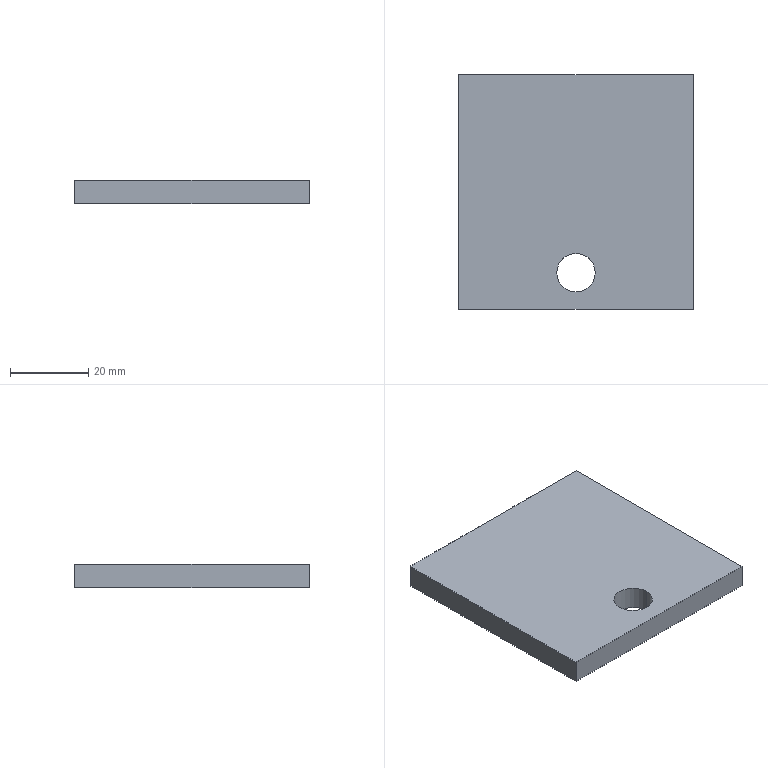Part | NX | features 凸台-拉伸21[2] 2 | 1 solid | 8 faces | box 60 x 60 x 6 mm | volume 21144 mm3 | plane 6 | cylinder 2 | commonest cylinder face diameters 9.834 x2
STEP:
#1=CARTESIAN_POINT('',(2758.083,-50.65,-1102.985));
#2=VERTEX_POINT('',#1);
#3=CARTESIAN_POINT('',(2758.083,-50.65,-1108.985));
#4=VERTEX_POINT('',#3);
#5=CARTESIAN_POINT('',(2758.083,-50.65,-1108.985));
#6=DIRECTION('',(0.,0.,1.));
#7=VECTOR('',#6,1000.);
#8=LINE('',#5,#7);
#9=EDGE_CURVE('',#2,#4,#8,.F.);
#10=ORIENTED_EDGE('',*,*,#9,.T.);
#11=CARTESIAN_POINT('',(2767.917,-50.65,-1108.985));
#12=VERTEX_POINT('',#11);
#13=CARTESIAN_POINT('',(2763.,-50.65,-1108.985));
#14=DIRECTION('',(0.,0.,-1.));
#15=DIRECTION('',(-1.,0.,0.));
#16=AXIS2_PLACEMENT_3D('',#13,#14,#15);
#17=CIRCLE('',#16,4.917);
#18=EDGE_CURVE('',#4,#12,#17,.T.);
#19=ORIENTED_EDGE('',*,*,#18,.T.);
#20=CARTESIAN_POINT('',(2767.917,-50.65,-1102.985));
#21=VERTEX_POINT('',#20);
#22=CARTESIAN_POINT('',(2767.917,-50.65,-1108.985));
#23=DIRECTION('',(0.,0.,1.));
#24=VECTOR('',#23,1000.);
#25=LINE('',#22,#24);
#26=EDGE_CURVE('',#12,#21,#25,.T.);
#27=ORIENTED_EDGE('',*,*,#26,.T.);
#28=CARTESIAN_POINT('',(2763.,-50.65,-1102.985));
#29=DIRECTION('',(0.,0.,-1.));
#30=DIRECTION('',(-1.,0.,0.));
#31=AXIS2_PLACEMENT_3D('',#28,#29,#30);
#32=CIRCLE('',#31,4.917);
#33=EDGE_CURVE('',#2,#21,#32,.T.);
#34=ORIENTED_EDGE('',*,*,#33,.F.);
#35=EDGE_LOOP('',(#10,#19,#27,#34));
#36=FACE_BOUND('',#35,.T.);
#37=CARTESIAN_POINT('',(2763.,-50.65,-1108.985));
#38=DIRECTION('',(0.,0.,1.));
#39=DIRECTION('',(1.,0.,0.));
#40=AXIS2_PLACEMENT_3D('',#37,#38,#39);
#41=CYLINDRICAL_SURFACE('',#40,4.917);
#42=ADVANCED_FACE('',(#36),#41,.F.);
#43=CARTESIAN_POINT('',(2733.,0.,-1102.985));
#44=VERTEX_POINT('',#43);
#45=CARTESIAN_POINT('',(2793.,0.,-1102.985));
#46=VERTEX_POINT('',#45);
#47=CARTESIAN_POINT('',(2793.,0.,-1102.985));
#48=DIRECTION('',(1.,0.,0.));
#49=VECTOR('',#48,1000.);
#50=LINE('',#47,#49);
#51=EDGE_CURVE('',#44,#46,#50,.T.);
#52=ORIENTED_EDGE('',*,*,#51,.T.);
#53=CARTESIAN_POINT('',(2793.,0.,-1108.985));
#54=VERTEX_POINT('',#53);
#55=CARTESIAN_POINT('',(2793.,0.,-1108.985));
#56=DIRECTION('',(0.,0.,1.));
#57=VECTOR('',#56,1000.);
#58=LINE('',#55,#57);
#59=EDGE_CURVE('',#54,#46,#58,.T.);
#60=ORIENTED_EDGE('',*,*,#59,.F.);
#61=CARTESIAN_POINT('',(2733.,0.,-1108.985));
#62=VERTEX_POINT('',#61);
#63=CARTESIAN_POINT('',(2793.,0.,-1108.985));
#64=DIRECTION('',(1.,0.,0.));
#65=VECTOR('',#64,1000.);
#66=LINE('',#63,#65);
#67=EDGE_CURVE('',#62,#54,#66,.T.);
#68=ORIENTED_EDGE('',*,*,#67,.F.);
#69=CARTESIAN_POINT('',(2733.,0.,-1108.985));
#70=DIRECTION('',(0.,0.,1.));
#71=VECTOR('',#70,1000.);
#72=LINE('',#69,#71);
#73=EDGE_CURVE('',#62,#44,#72,.T.);
#74=ORIENTED_EDGE('',*,*,#73,.T.);
#75=EDGE_LOOP('',(#52,#60,#68,#74));
#76=FACE_BOUND('',#75,.T.);
#77=CARTESIAN_POINT('',(2793.,0.,-1108.985));
#78=DIRECTION('',(0.,-1.,0.));
#79=DIRECTION('',(1.,0.,0.));
#80=AXIS2_PLACEMENT_3D('',#77,#78,#79);
#81=PLANE('',#80);
#82=ADVANCED_FACE('',(#76),#81,.F.);
#83=CARTESIAN_POINT('',(2733.,-60.,-1102.985));
#84=VERTEX_POINT('',#83);
#85=CARTESIAN_POINT('',(2733.,0.,-1102.985));
#86=DIRECTION('',(0.,1.,0.));
#87=VECTOR('',#86,1000.);
#88=LINE('',#85,#87);
#89=EDGE_CURVE('',#84,#44,#88,.T.);
#90=ORIENTED_EDGE('',*,*,#89,.T.);
#91=ORIENTED_EDGE('',*,*,#73,.F.);
#92=CARTESIAN_POINT('',(2733.,-60.,-1108.985));
#93=VERTEX_POINT('',#92);
#94=CARTESIAN_POINT('',(2733.,0.,-1108.985));
#95=DIRECTION('',(0.,1.,0.));
#96=VECTOR('',#95,1000.);
#97=LINE('',#94,#96);
#98=EDGE_CURVE('',#93,#62,#97,.T.);
#99=ORIENTED_EDGE('',*,*,#98,.F.);
#100=CARTESIAN_POINT('',(2733.,-60.,-1108.985));
#101=DIRECTION('',(0.,0.,1.));
#102=VECTOR('',#101,1000.);
#103=LINE('',#100,#102);
#104=EDGE_CURVE('',#93,#84,#103,.T.);
#105=ORIENTED_EDGE('',*,*,#104,.T.);
#106=EDGE_LOOP('',(#90,#91,#99,#105));
#107=FACE_BOUND('',#106,.T.);
#108=CARTESIAN_POINT('',(2733.,0.,-1108.985));
#109=DIRECTION('',(1.,0.,0.));
#110=DIRECTION('',(0.,0.,-1.));
#111=AXIS2_PLACEMENT_3D('',#108,#109,#110);
#112=PLANE('',#111);
#113=ADVANCED_FACE('',(#107),#112,.F.);
#114=CARTESIAN_POINT('',(2793.,-60.,-1102.985));
#115=VERTEX_POINT('',#114);
#116=CARTESIAN_POINT('',(2793.,-60.,-1102.985));
#117=DIRECTION('',(-1.,0.,0.));
#118=VECTOR('',#117,1000.);
#119=LINE('',#116,#118);
#120=EDGE_CURVE('',#115,#84,#119,.T.);
#121=ORIENTED_EDGE('',*,*,#120,.T.);
#122=ORIENTED_EDGE('',*,*,#104,.F.);
#123=CARTESIAN_POINT('',(2793.,-60.,-1108.985));
#124=VERTEX_POINT('',#123);
#125=CARTESIAN_POINT('',(2793.,-60.,-1108.985));
#126=DIRECTION('',(-1.,0.,0.));
#127=VECTOR('',#126,1000.);
#128=LINE('',#125,#127);
#129=EDGE_CURVE('',#124,#93,#128,.T.);
#130=ORIENTED_EDGE('',*,*,#129,.F.);
#131=CARTESIAN_POINT('',(2793.,-60.,-1108.985));
#132=DIRECTION('',(0.,0.,1.));
#133=VECTOR('',#132,1000.);
#134=LINE('',#131,#133);
#135=EDGE_CURVE('',#124,#115,#134,.T.);
#136=ORIENTED_EDGE('',*,*,#135,.T.);
#137=EDGE_LOOP('',(#121,#122,#130,#136));
#138=FACE_BOUND('',#137,.T.);
#139=CARTESIAN_POINT('',(2793.,-60.,-1108.985));
#140=DIRECTION('',(0.,1.,0.));
#141=DIRECTION('',(0.,0.,1.));
#142=AXIS2_PLACEMENT_3D('',#139,#140,#141);
#143=PLANE('',#142);
#144=ADVANCED_FACE('',(#138),#143,.F.);
#145=CARTESIAN_POINT('',(2793.,0.,-1102.985));
#146=DIRECTION('',(0.,-1.,0.));
#147=VECTOR('',#146,1000.);
#148=LINE('',#145,#147);
#149=EDGE_CURVE('',#46,#115,#148,.T.);
#150=ORIENTED_EDGE('',*,*,#149,.T.);
#151=ORIENTED_EDGE('',*,*,#135,.F.);
#152=CARTESIAN_POINT('',(2793.,0.,-1108.985));
#153=DIRECTION('',(0.,-1.,0.));
#154=VECTOR('',#153,1000.);
#155=LINE('',#152,#154);
#156=EDGE_CURVE('',#54,#124,#155,.T.);
#157=ORIENTED_EDGE('',*,*,#156,.F.);
#158=ORIENTED_EDGE('',*,*,#59,.T.);
#159=EDGE_LOOP('',(#150,#151,#157,#158));
#160=FACE_BOUND('',#159,.T.);
#161=CARTESIAN_POINT('',(2793.,0.,-1108.985));
#162=DIRECTION('',(-1.,0.,0.));
#163=DIRECTION('',(0.,-1.,0.));
#164=AXIS2_PLACEMENT_3D('',#161,#162,#163);
#165=PLANE('',#164);
#166=ADVANCED_FACE('',(#160),#165,.F.);
#167=CARTESIAN_POINT('',(2763.,-50.65,-1102.985));
#168=DIRECTION('',(0.,0.,-1.));
#169=DIRECTION('',(-1.,0.,0.));
#170=AXIS2_PLACEMENT_3D('',#167,#168,#169);
#171=CIRCLE('',#170,4.917);
#172=EDGE_CURVE('',#21,#2,#171,.T.);
#173=ORIENTED_EDGE('',*,*,#172,.T.);
#174=ORIENTED_EDGE('',*,*,#33,.T.);
#175=EDGE_LOOP('',(#173,#174));
#176=FACE_BOUND('',#175,.T.);
#177=ORIENTED_EDGE('',*,*,#149,.F.);
#178=ORIENTED_EDGE('',*,*,#51,.F.);
#179=ORIENTED_EDGE('',*,*,#89,.F.);
#180=ORIENTED_EDGE('',*,*,#120,.F.);
#181=EDGE_LOOP('',(#177,#178,#179,#180));
#182=FACE_BOUND('',#181,.T.);
#183=CARTESIAN_POINT('',(1500.,0.,-1102.985));
#184=DIRECTION('',(0.,0.,-1.));
#185=DIRECTION('',(-1.,0.,0.));
#186=AXIS2_PLACEMENT_3D('',#183,#184,#185);
#187=PLANE('',#186);
#188=ADVANCED_FACE('',(#176,#182),#187,.F.);
#189=CARTESIAN_POINT('',(2763.,-50.65,-1108.985));
#190=DIRECTION('',(0.,0.,-1.));
#191=DIRECTION('',(-1.,0.,0.));
#192=AXIS2_PLACEMENT_3D('',#189,#190,#191);
#193=CIRCLE('',#192,4.917);
#194=EDGE_CURVE('',#12,#4,#193,.T.);
#195=ORIENTED_EDGE('',*,*,#194,.F.);
#196=ORIENTED_EDGE('',*,*,#18,.F.);
#197=EDGE_LOOP('',(#195,#196));
#198=FACE_BOUND('',#197,.T.);
#199=ORIENTED_EDGE('',*,*,#156,.T.);
#200=ORIENTED_EDGE('',*,*,#129,.T.);
#201=ORIENTED_EDGE('',*,*,#98,.T.);
#202=ORIENTED_EDGE('',*,*,#67,.T.);
#203=EDGE_LOOP('',(#199,#200,#201,#202));
#204=FACE_BOUND('',#203,.T.);
#205=CARTESIAN_POINT('',(1500.,0.,-1108.985));
#206=DIRECTION('',(0.,0.,-1.));
#207=DIRECTION('',(-1.,0.,0.));
#208=AXIS2_PLACEMENT_3D('',#205,#206,#207);
#209=PLANE('',#208);
#210=ADVANCED_FACE('',(#198,#204),#209,.T.);
#211=ORIENTED_EDGE('',*,*,#194,.T.);
#212=ORIENTED_EDGE('',*,*,#9,.F.);
#213=ORIENTED_EDGE('',*,*,#172,.F.);
#214=ORIENTED_EDGE('',*,*,#26,.F.);
#215=EDGE_LOOP('',(#211,#212,#213,#214));
#216=FACE_BOUND('',#215,.T.);
#217=CARTESIAN_POINT('',(2763.,-50.65,-1108.985));
#218=DIRECTION('',(0.,0.,1.));
#219=DIRECTION('',(1.,0.,0.));
#220=AXIS2_PLACEMENT_3D('',#217,#218,#219);
#221=CYLINDRICAL_SURFACE('',#220,4.917);
#222=ADVANCED_FACE('',(#216),#221,.F.);
#223=CLOSED_SHELL('',(#42,#82,#113,#144,#166,#188,#210,#222));
#224=MANIFOLD_SOLID_BREP('',#223);
#225=(LENGTH_UNIT()NAMED_UNIT(*)SI_UNIT(.MILLI.,.METRE.));
#226=UNCERTAINTY_MEASURE_WITH_UNIT(LENGTH_MEASURE(0.00001),#225,'','');
#227=(NAMED_UNIT(*)PLANE_ANGLE_UNIT()SI_UNIT($,.RADIAN.));
#228=(NAMED_UNIT(*)SI_UNIT($,.STERADIAN.)SOLID_ANGLE_UNIT());
#229=(GEOMETRIC_REPRESENTATION_CONTEXT(3)GLOBAL_UNCERTAINTY_ASSIGNED_CONTEXT((#226))GLOBAL_UNIT_ASSIGNED_CONTEXT((#225,#227,#228))REPRESENTATION_CONTEXT('',''));
#230=ADVANCED_BREP_SHAPE_REPRESENTATION('',(#224),#229);